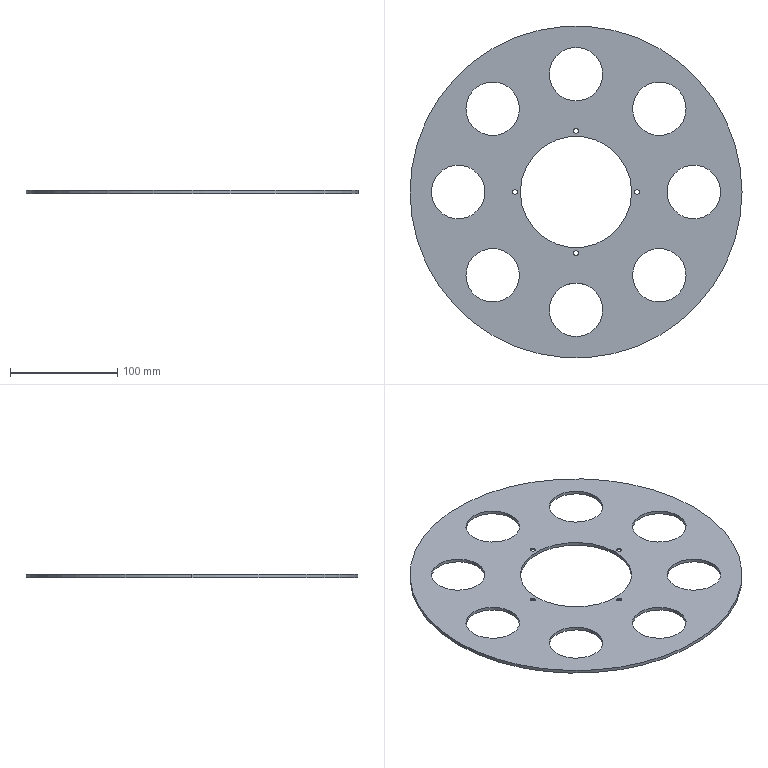Part | STEP file | 2007 Limit side plate A | 1 solid | 38 faces | box 310 x 310 x 3 mm | volume 153476 mm3 | cylinder 28 | cone 8 | plane 2 | commonest cylinder face diameters 50 x16 4.5 x8 104 x2 310 x2